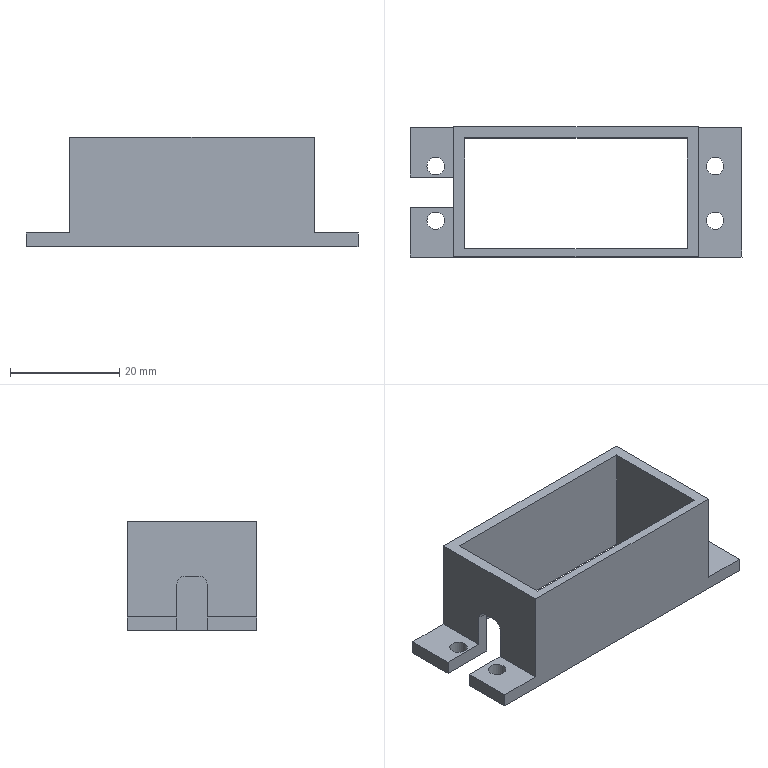Part | STEP file | Wytnij-wyci_gni_cie2_3 | 1 solid | 25 faces | box 60.8 x 23.8 x 20 mm | volume 5414 mm3 | plane 19 | cylinder 6 | commonest cylinder face diameters 3.2 x4 3 x2